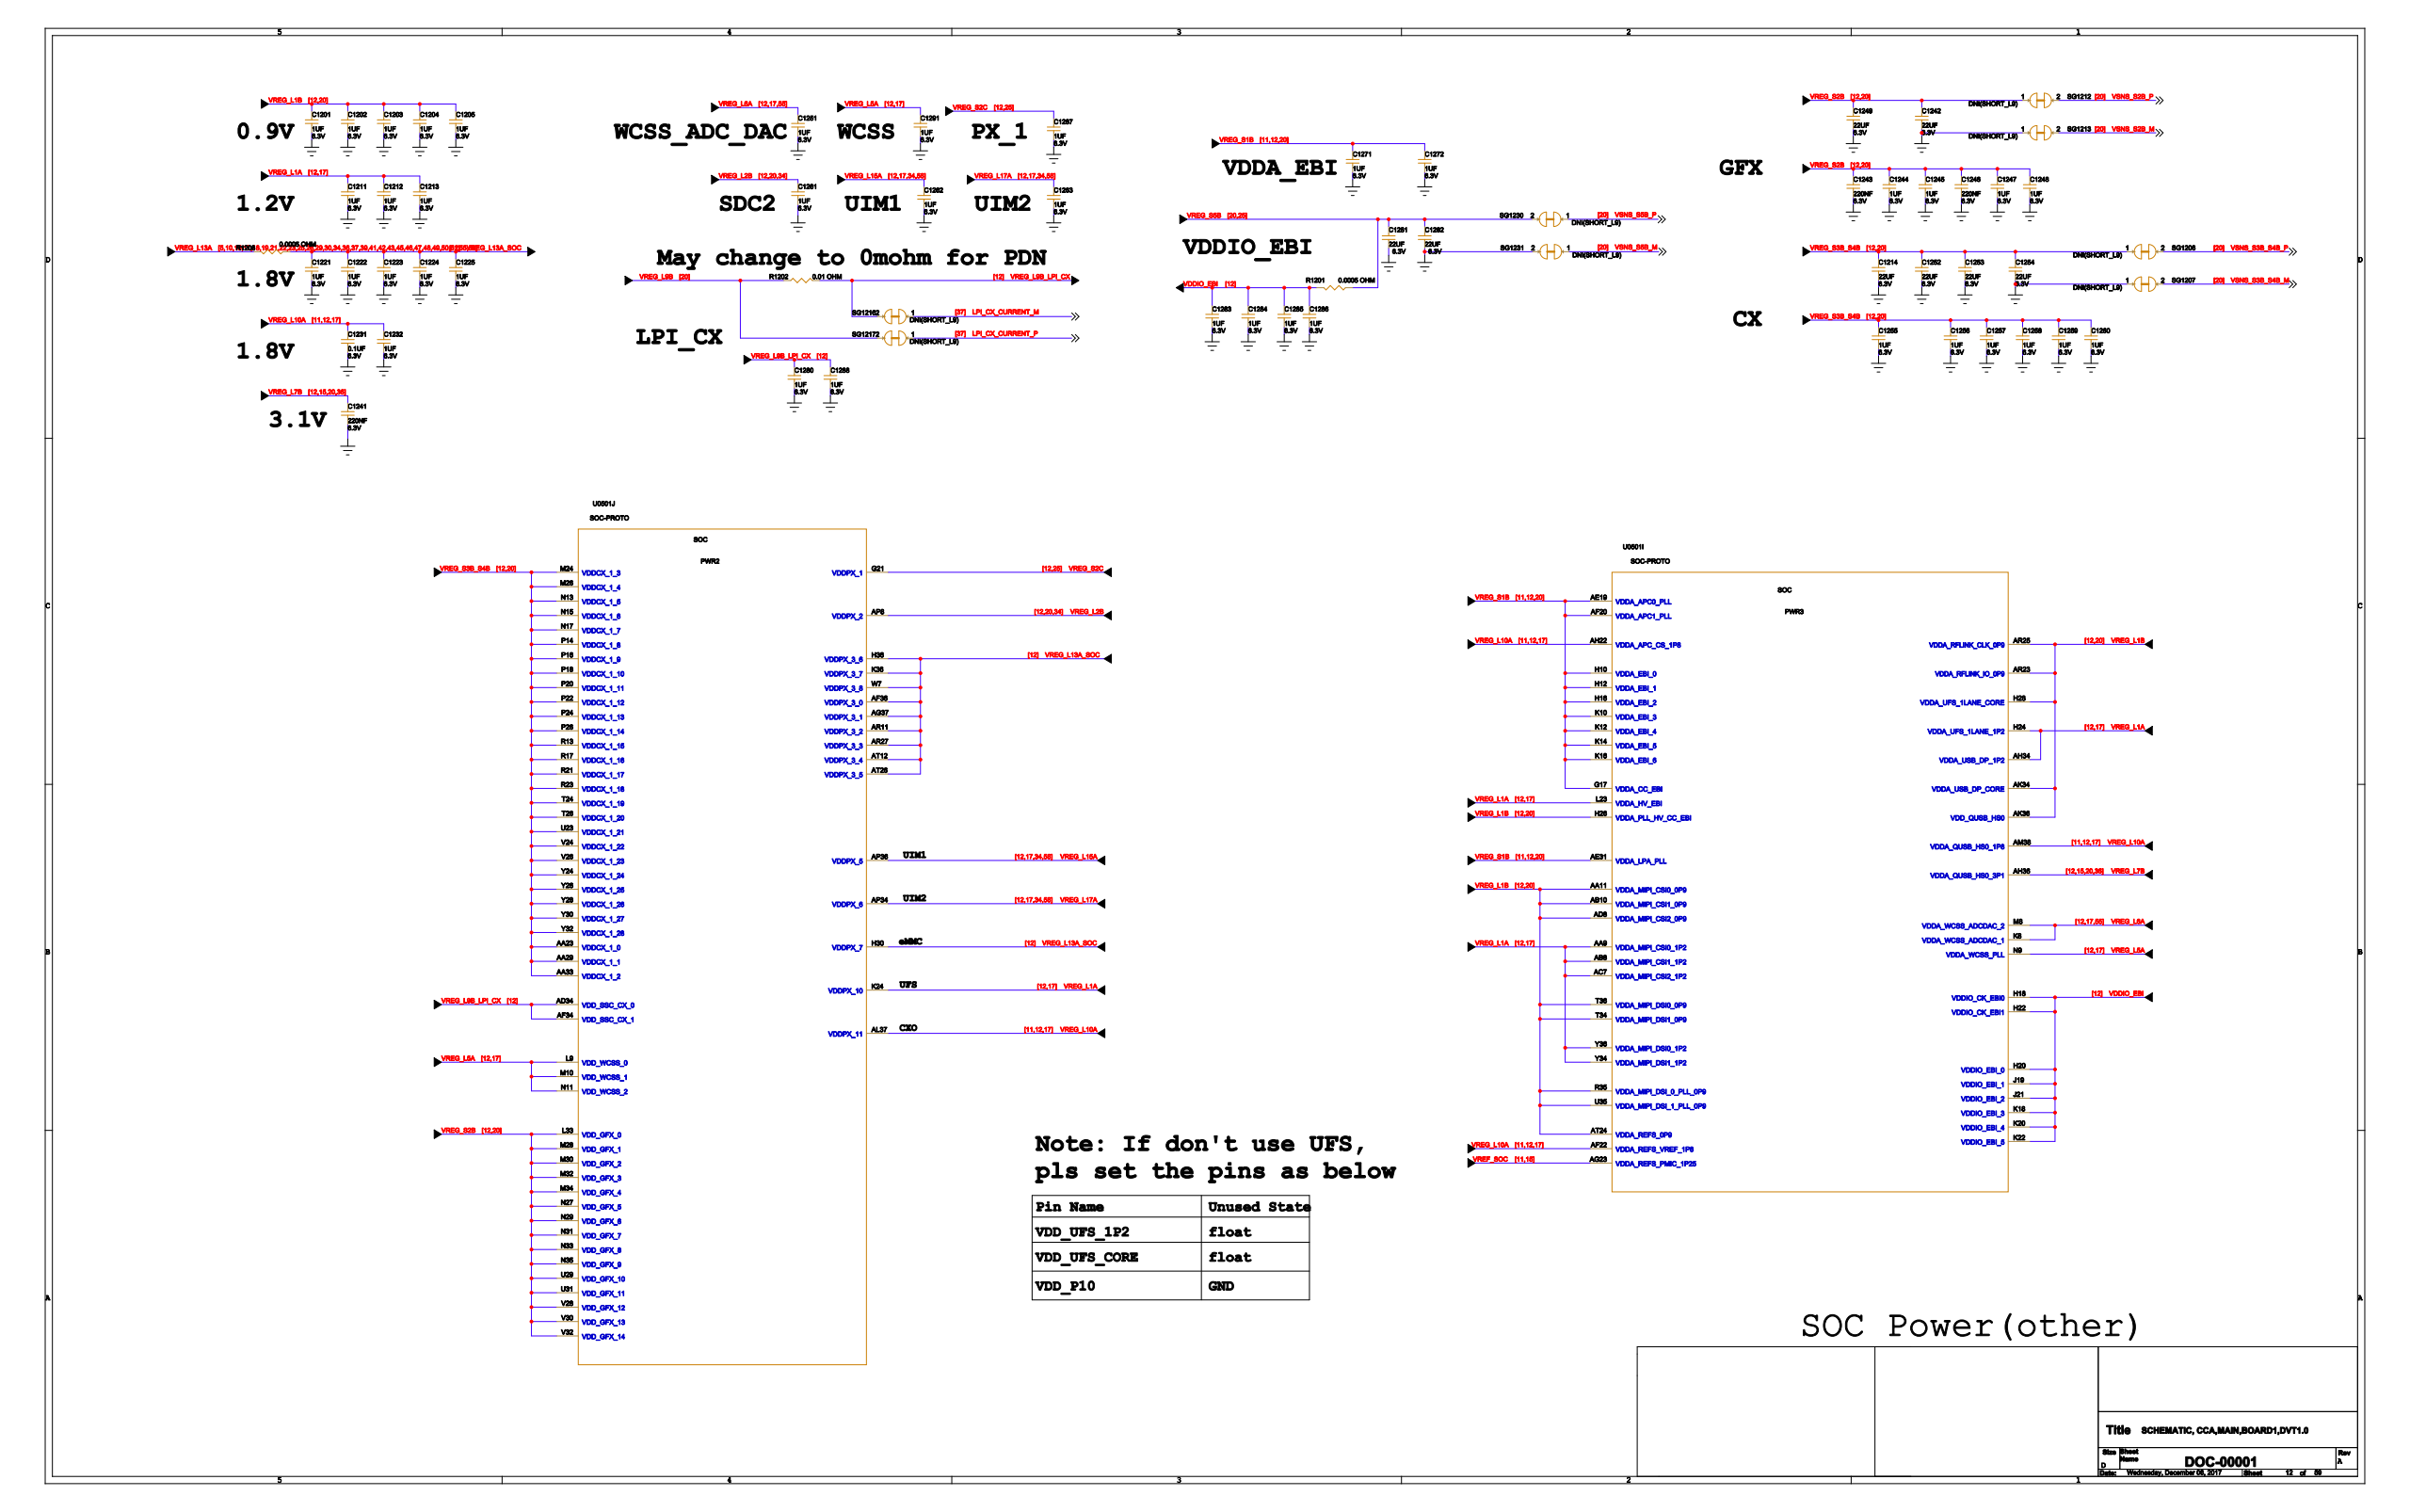Circuit board | KiCad | 1657 parts | 1365 nets | one sheet of the schematic
Parts on this sheet (reference | value | footprint):
C1201
C1202
C1203
C1204
C1205
C1211
C1212
C1213
C1214
C1221
C1222
C1223
C1224
C1225
C1231
C1232
C1241
C1242
C1243
C1244
C1245
C1246
C1247
C1248
C1249
C1251
C1252
C1253
C1254
C1255
C1256
C1257
C1258
C1259
C1260
C1261
C1262
C1263
C1271
C1272
C1280
C1281
C1282
C1283
C1284
C1285
C1286
C1287
C1288
C1291
R1201
R1202
R1208
SG1206
SG1207
SG1212
SG1213
SG1216
SG1217
SG1230
SG1231
U0501
Nets of these parts (net: part-pin ...):
GND: C1201-2 C1202-2 C1203-2 C1204-2 C1205-2 C1211-2 C1212-2 C1213-2 C1214-2 C1221-2 C1222-2 C1223-2 C1224-2 C1225-2 C1231-2 C1232-2 C1241-2 C1242-2 C1243-2 C1244-2 C1245-2 C1246-2 C1247-2 C1248-2 C1249-2 C1251-2 C1252-2 C1253-2 C1254-2 C1255-2 C1256-2 C1257-2 C1258-2 C1259-2 C1260-2 C1261-2 C1262-2 C1263-2 C1271-2 C1272-2 C1280-2 C1281-1 C1282-1 C1283-2 C1284-2 C1285-2 C1286-2 C1287-2 C1288-2 C1291-2 SG1207-1 SG1213-1 SG1231-2
VREG_L13A: R1208-2
VREG_L2B: C1261-1 U0501-AP8
VSNS_S3B_S4B_M: SG1207-2
VREG_S2C: C1287-1 U0501-G21
VREG_S2B: C1242-1 C1243-1 C1244-1 C1245-1 C1246-1 C1247-1 C1248-1 C1249-1 SG1212-1 U0501-L33 U0501-M28 U0501-M30 U0501-M32 U0501-M34 U0501-N27 U0501-N29 U0501-N31 U0501-N33 U0501-N35 U0501-U29 U0501-U31 U0501-V28 U0501-V30 U0501-V32
VSNS_S2B_P: SG1212-2
VREG_L7B: C1241-1 U0501-AH36
VREG_L17A: C1263-1 U0501-AP34
VREG_S3B_S4B: C1214-1 C1252-1 C1253-1 C1254-1 C1255-1 C1256-1 C1257-1 C1258-1 C1259-1 C1260-1 SG1206-1 U0501-AA23 U0501-AA29 U0501-AA33 U0501-M24 U0501-M26 U0501-N13 U0501-N15 U0501-N17 U0501-P14 U0501-P16 U0501-P18 U0501-P20 U0501-P22 U0501-P24 U0501-P26 U0501-R13 U0501-R17 U0501-R21 U0501-R23 U0501-T24 U0501-T26 U0501-U23 U0501-V24 U0501-V26 U0501-Y24 U0501-Y26 U0501-Y28 U0501-Y30 U0501-Y32
VSNS_S5B_M: SG1231-1
VSNS_S2B_M: SG1213-2
VREG_L15A: C1262-1 U0501-AP36
VREG_L1A: C1211-1 C1212-1 C1213-1 U0501-AA9 U0501-AB8 U0501-AC7 U0501-AH34 U0501-H24 U0501-K24 U0501-L23 U0501-Y34 U0501-Y36
VREG_L1B: C1201-1 C1202-1 C1203-1 C1204-1 C1205-1 U0501-AA11 U0501-AB10 U0501-AD8 U0501-AK34 U0501-AK36 U0501-AR23 U0501-AR25 U0501-AT24 U0501-H26 U0501-H28 U0501-R35 U0501-T34 U0501-T36 U0501-U35
VREG_S1B: C1271-1 C1272-1 U0501-AE19 U0501-AE31 U0501-AF20 U0501-G17 U0501-H10 U0501-H12 U0501-H16 U0501-K10 U0501-K12 U0501-K14 U0501-K16
REG_L9B_LPI_CX: C1280-1 C1288-1 R1202-1 SG1216-2 U0501-AD34 U0501-AF34
VREG_L10A: C1231-1 C1232-1 U0501-AF22 U0501-AH22 U0501-AL37 U0501-AM38
VREG_L13A_SOC: C1221-1 C1222-1 C1223-1 C1224-1 C1225-1 R1208-1 U0501-AF36 U0501-AG37 U0501-AR11 U0501-AR27 U0501-AT12 U0501-AT26 U0501-H30 U0501-H36 U0501-K36 U0501-W7
VREF_SOC: U0501-AG23
VDDIO_EBI: C1283-1 C1284-1 C1285-1 C1286-1 R1201-1 U0501-H18 U0501-H20 U0501-H22 U0501-J19 U0501-J21 U0501-K18 U0501-K20 U0501-K22
VREG_L6A: C1251-1 U0501-K8 U0501-M8
VREG_L5A: C1291-1 U0501-L9 U0501-M10 U0501-N9 U0501-N11
VREG_S5B: C1281-2 C1282-2 R1201-2 SG1230-2
I_CX_CURRENT_M: SG1216-1
VSNS_S3B_S4B_P: SG1206-2
I_CX_CURRENT_P: SG1217-1
VREG_L9B: R1202-2 SG1217-2
VSNS_S5B_P: SG1230-1